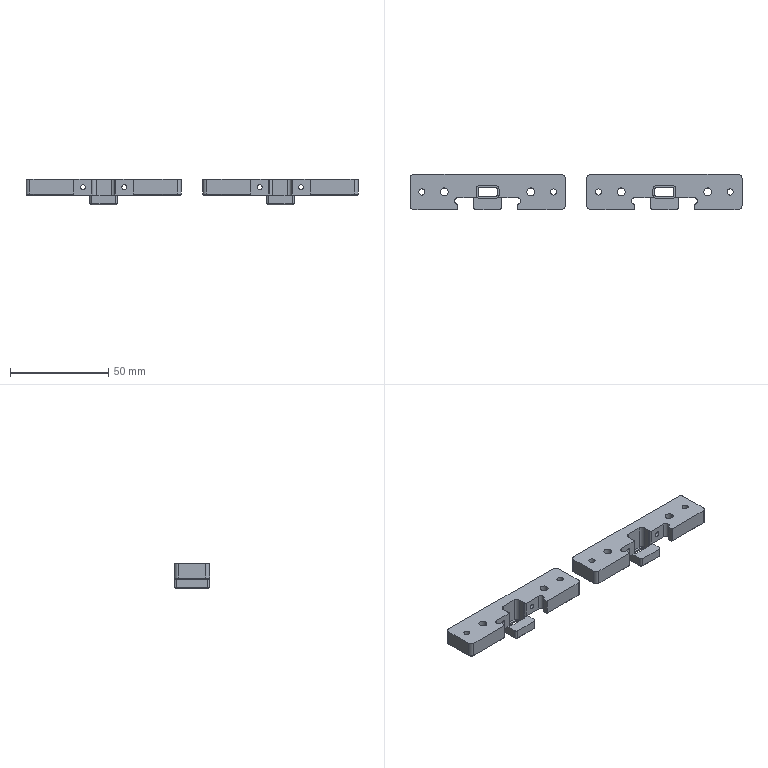Part | 2 solids | 164 faces | box 169 x 18 x 12.9 mm | volume 18939 mm3 | plane 76 | cylinder 72 | cone 16 | commonest cylinder face diameters 2 x16 4 x16 2.5 x8 3.1 x8 4.1 x8 6 x8